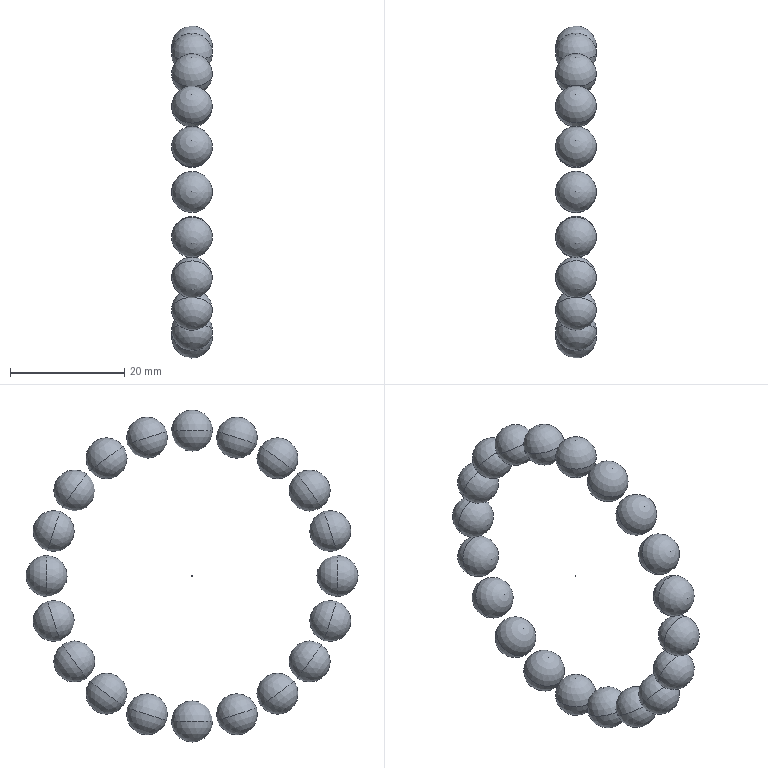Part | STEP file | bearing_6908_03V11 | 21 solids | 42 faces | box 7.2 x 58.195 x 58.195 mm | volume 3909 mm3 | sphere 42